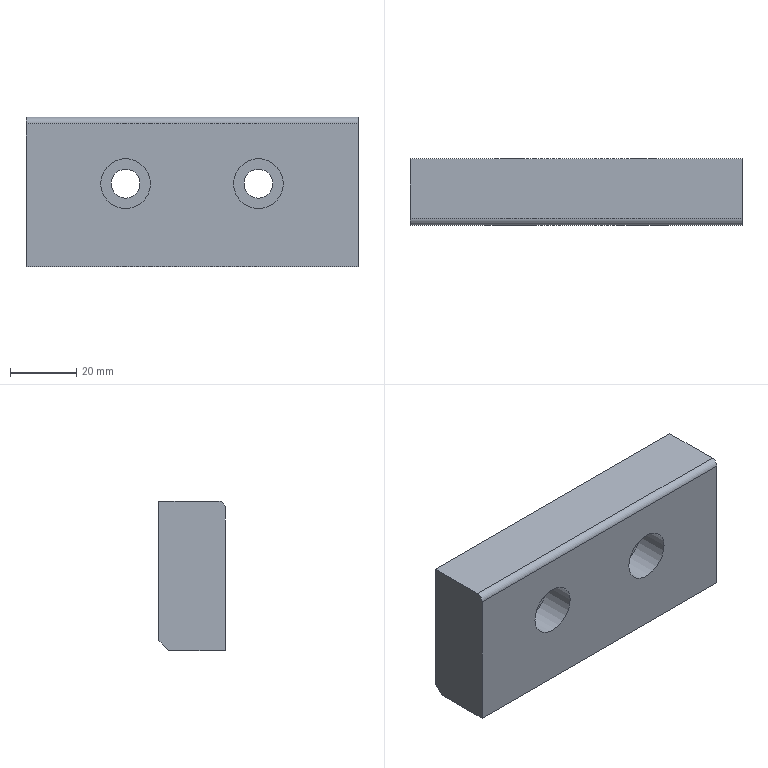Part | STEP file | 1_id1578_x_t | 1 solid | 14 faces | box 100 x 20 x 45 mm | volume 84741 mm3 | plane 9 | cylinder 5 | commonest cylinder face diameters 8.7 x2 15 x2 4 x1
STEP:
#1=CARTESIAN_POINT('',(0.,0.,0.));
#2=DIRECTION('',(0.,0.,1.));
#3=DIRECTION('',(1.,0.,0.));
#4=AXIS2_PLACEMENT_3D('',#1,#2,#3);
#5=CARTESIAN_POINT('',(797.926,444.972,-87.248));
#6=VERTEX_POINT('',#5);
#7=CARTESIAN_POINT('',(697.926,444.972,-87.248));
#8=VERTEX_POINT('',#7);
#9=CARTESIAN_POINT('',(797.926,444.972,-87.248));
#10=DIRECTION('',(-1.,0.,0.));
#11=VECTOR('',#10,1.);
#12=LINE('',#9,#11);
#13=CARTESIAN_POINT('',(707.926,444.972,-87.248));
#14=DIRECTION('',(0.,0.7071,-0.7071));
#15=DIRECTION('',(0.,-0.7071,-0.7071));
#16=AXIS2_PLACEMENT_3D('',#13,#14,#15);
#17=PLANE('',#16);
#18=CARTESIAN_POINT('',(0.,-90.));
#19=DIRECTION('',(0.,1.));
#20=VECTOR('',#19,1.);
#21=LINE('',#18,#20);
#22=(GEOMETRIC_REPRESENTATION_CONTEXT(2)PARAMETRIC_REPRESENTATION_CONTEXT()REPRESENTATION_CONTEXT('',''));
#23=DEFINITIONAL_REPRESENTATION('',(#21),#22);
#24=PCURVE('',#17,#23);
#25=CARTESIAN_POINT('',(707.926,444.972,-107.548));
#26=DIRECTION('',(0.,1.,0.));
#27=DIRECTION('',(1.,0.,0.));
#28=AXIS2_PLACEMENT_3D('',#25,#26,#27);
#29=PLANE('',#28);
#30=CARTESIAN_POINT('',(90.,-20.3));
#31=DIRECTION('',(-1.,0.));
#32=VECTOR('',#31,1.);
#33=LINE('',#30,#32);
#34=(GEOMETRIC_REPRESENTATION_CONTEXT(2)PARAMETRIC_REPRESENTATION_CONTEXT()REPRESENTATION_CONTEXT('',''));
#35=DEFINITIONAL_REPRESENTATION('',(#33),#34);
#36=PCURVE('',#29,#35);
#37=SURFACE_CURVE('',#12,(#24,#36),.PCURVE_S1.);
#38=EDGE_CURVE('',#6,#8,#37,.T.);
#39=ORIENTED_EDGE('',*,*,#38,.F.);
#40=CARTESIAN_POINT('',(797.926,441.972,-90.248));
#41=VERTEX_POINT('',#40);
#42=CARTESIAN_POINT('',(797.926,441.972,-90.248));
#43=DIRECTION('',(0.,0.7071,0.7071));
#44=VECTOR('',#43,1.);
#45=LINE('',#42,#44);
#46=CARTESIAN_POINT('',(4.243,-90.));
#47=DIRECTION('',(-1.,0.));
#48=VECTOR('',#47,1.);
#49=LINE('',#46,#48);
#50=(GEOMETRIC_REPRESENTATION_CONTEXT(2)PARAMETRIC_REPRESENTATION_CONTEXT()REPRESENTATION_CONTEXT('',''));
#51=DEFINITIONAL_REPRESENTATION('',(#49),#50);
#52=PCURVE('',#17,#51);
#53=CARTESIAN_POINT('',(797.926,544.972,-45.248));
#54=DIRECTION('',(-1.,0.,0.));
#55=DIRECTION('',(0.,0.,-1.));
#56=AXIS2_PLACEMENT_3D('',#53,#54,#55);
#57=PLANE('',#56);
#58=CARTESIAN_POINT('',(45.,103.));
#59=DIRECTION('',(-0.7071,-0.7071));
#60=VECTOR('',#59,1.);
#61=LINE('',#58,#60);
#62=(GEOMETRIC_REPRESENTATION_CONTEXT(2)PARAMETRIC_REPRESENTATION_CONTEXT()REPRESENTATION_CONTEXT('',''));
#63=DEFINITIONAL_REPRESENTATION('',(#61),#62);
#64=PCURVE('',#57,#63);
#65=SURFACE_CURVE('',#45,(#52,#64),.PCURVE_S1.);
#66=EDGE_CURVE('',#41,#6,#65,.T.);
#67=ORIENTED_EDGE('',*,*,#66,.F.);
#68=CARTESIAN_POINT('',(697.926,441.972,-90.248));
#69=VERTEX_POINT('',#68);
#70=CARTESIAN_POINT('',(697.926,441.972,-90.248));
#71=DIRECTION('',(1.,0.,0.));
#72=VECTOR('',#71,1.);
#73=LINE('',#70,#72);
#74=CARTESIAN_POINT('',(4.243,10.));
#75=DIRECTION('',(0.,-1.));
#76=VECTOR('',#75,1.);
#77=LINE('',#74,#76);
#78=(GEOMETRIC_REPRESENTATION_CONTEXT(2)PARAMETRIC_REPRESENTATION_CONTEXT()REPRESENTATION_CONTEXT('',''));
#79=DEFINITIONAL_REPRESENTATION('',(#77),#78);
#80=PCURVE('',#17,#79);
#81=CARTESIAN_POINT('',(787.926,424.972,-90.248));
#82=DIRECTION('',(0.,0.,1.));
#83=DIRECTION('',(-1.,0.,0.));
#84=AXIS2_PLACEMENT_3D('',#81,#82,#83);
#85=PLANE('',#84);
#86=CARTESIAN_POINT('',(90.,-17.));
#87=DIRECTION('',(-1.,0.));
#88=VECTOR('',#87,1.);
#89=LINE('',#86,#88);
#90=(GEOMETRIC_REPRESENTATION_CONTEXT(2)PARAMETRIC_REPRESENTATION_CONTEXT()REPRESENTATION_CONTEXT('',''));
#91=DEFINITIONAL_REPRESENTATION('',(#89),#90);
#92=PCURVE('',#85,#91);
#93=SURFACE_CURVE('',#73,(#80,#92),.PCURVE_S1.);
#94=EDGE_CURVE('',#69,#41,#93,.T.);
#95=ORIENTED_EDGE('',*,*,#94,.F.);
#96=CARTESIAN_POINT('',(697.926,444.972,-87.248));
#97=DIRECTION('',(0.,-0.7071,-0.7071));
#98=VECTOR('',#97,1.);
#99=LINE('',#96,#98);
#100=CARTESIAN_POINT('',(0.,10.));
#101=DIRECTION('',(1.,0.));
#102=VECTOR('',#101,1.);
#103=LINE('',#100,#102);
#104=(GEOMETRIC_REPRESENTATION_CONTEXT(2)PARAMETRIC_REPRESENTATION_CONTEXT()REPRESENTATION_CONTEXT('',''));
#105=DEFINITIONAL_REPRESENTATION('',(#103),#104);
#106=PCURVE('',#17,#105);
#107=CARTESIAN_POINT('',(697.926,444.972,-45.248));
#108=DIRECTION('',(1.,0.,0.));
#109=DIRECTION('',(0.,0.,-1.));
#110=AXIS2_PLACEMENT_3D('',#107,#108,#109);
#111=PLANE('',#110);
#112=CARTESIAN_POINT('',(42.,0.));
#113=DIRECTION('',(0.7071,-0.7071));
#114=VECTOR('',#113,1.);
#115=LINE('',#112,#114);
#116=(GEOMETRIC_REPRESENTATION_CONTEXT(2)PARAMETRIC_REPRESENTATION_CONTEXT()REPRESENTATION_CONTEXT('',''));
#117=DEFINITIONAL_REPRESENTATION('',(#115),#116);
#118=PCURVE('',#111,#117);
#119=SURFACE_CURVE('',#99,(#106,#118),.PCURVE_S1.);
#120=EDGE_CURVE('',#8,#69,#119,.T.);
#121=ORIENTED_EDGE('',*,*,#120,.F.);
#122=EDGE_LOOP('',(#39,#67,#95,#121));
#123=FACE_BOUND('',#122,.T.);
#124=ADVANCED_FACE('',(#123),#17,.T.);
#125=CARTESIAN_POINT('',(697.926,424.972,-47.248));
#126=VERTEX_POINT('',#125);
#127=CARTESIAN_POINT('',(697.926,424.972,-90.248));
#128=VERTEX_POINT('',#127);
#129=CARTESIAN_POINT('',(697.926,424.972,-47.248));
#130=DIRECTION('',(0.,0.,-1.));
#131=VECTOR('',#130,1.);
#132=LINE('',#129,#131);
#133=CARTESIAN_POINT('',(2.,-20.));
#134=DIRECTION('',(1.,0.));
#135=VECTOR('',#134,1.);
#136=LINE('',#133,#135);
#137=(GEOMETRIC_REPRESENTATION_CONTEXT(2)PARAMETRIC_REPRESENTATION_CONTEXT()REPRESENTATION_CONTEXT('',''));
#138=DEFINITIONAL_REPRESENTATION('',(#136),#137);
#139=PCURVE('',#111,#138);
#140=CARTESIAN_POINT('',(787.926,424.972,-107.548));
#141=DIRECTION('',(0.,-1.,0.));
#142=DIRECTION('',(-1.,0.,0.));
#143=AXIS2_PLACEMENT_3D('',#140,#141,#142);
#144=PLANE('',#143);
#145=CARTESIAN_POINT('',(90.,-60.3));
#146=DIRECTION('',(0.,1.));
#147=VECTOR('',#146,1.);
#148=LINE('',#145,#147);
#149=(GEOMETRIC_REPRESENTATION_CONTEXT(2)PARAMETRIC_REPRESENTATION_CONTEXT()REPRESENTATION_CONTEXT('',''));
#150=DEFINITIONAL_REPRESENTATION('',(#148),#149);
#151=PCURVE('',#144,#150);
#152=SURFACE_CURVE('',#132,(#139,#151),.PCURVE_S1.);
#153=EDGE_CURVE('',#126,#128,#152,.T.);
#154=ORIENTED_EDGE('',*,*,#153,.F.);
#155=CARTESIAN_POINT('',(697.926,426.972,-45.248));
#156=VERTEX_POINT('',#155);
#157=CARTESIAN_POINT('',(697.926,426.972,-47.248));
#158=DIRECTION('',(-1.,0.,0.));
#159=DIRECTION('',(0.,-1.,0.));
#160=AXIS2_PLACEMENT_3D('',#157,#158,#159);
#161=CIRCLE('',#160,2.);
#162=CARTESIAN_POINT('',(2.,-20.));
#163=CARTESIAN_POINT('',(-1.464,-20.));
#164=CARTESIAN_POINT('',(0.2679,-17.));
#165=CARTESIAN_POINT('',(2.,-14.));
#166=CARTESIAN_POINT('',(3.732,-17.));
#167=CARTESIAN_POINT('',(5.464,-20.));
#168=CARTESIAN_POINT('',(2.,-20.));
#169=(BOUNDED_CURVE()B_SPLINE_CURVE(2,(#162,#163,#164,#165,#166,#167,#168),.UNSPECIFIED.,.T.,.F.)B_SPLINE_CURVE_WITH_KNOTS((1,2,2,2,2,1),(-2.094,0.,2.094,4.189,6.283,8.378),.UNSPECIFIED.)CURVE()GEOMETRIC_REPRESENTATION_ITEM()RATIONAL_B_SPLINE_CURVE((1.,0.5,1.,0.5,1.,0.5,1.))REPRESENTATION_ITEM(''));
#170=(GEOMETRIC_REPRESENTATION_CONTEXT(2)PARAMETRIC_REPRESENTATION_CONTEXT()REPRESENTATION_CONTEXT('',''));
#171=DEFINITIONAL_REPRESENTATION('',(#169),#170);
#172=PCURVE('',#111,#171);
#173=CARTESIAN_POINT('',(787.926,426.972,-47.248));
#174=DIRECTION('',(1.,0.,0.));
#175=DIRECTION('',(0.,1.,0.));
#176=AXIS2_PLACEMENT_3D('',#173,#174,#175);
#177=CYLINDRICAL_SURFACE('',#176,2.);
#178=CARTESIAN_POINT('',(3.142,-90.));
#179=DIRECTION('',(-1.,0.));
#180=VECTOR('',#179,1.);
#181=LINE('',#178,#180);
#182=(GEOMETRIC_REPRESENTATION_CONTEXT(2)PARAMETRIC_REPRESENTATION_CONTEXT()REPRESENTATION_CONTEXT('',''));
#183=DEFINITIONAL_REPRESENTATION('',(#181),#182);
#184=PCURVE('',#177,#183);
#185=SURFACE_CURVE('',#161,(#172,#184),.PCURVE_S1.);
#186=EDGE_CURVE('',#126,#156,#185,.T.);
#187=ORIENTED_EDGE('',*,*,#186,.T.);
#188=CARTESIAN_POINT('',(697.926,444.972,-45.248));
#189=VERTEX_POINT('',#188);
#190=CARTESIAN_POINT('',(697.926,444.972,-45.248));
#191=DIRECTION('',(0.,-1.,0.));
#192=VECTOR('',#191,1.);
#193=LINE('',#190,#192);
#194=CARTESIAN_POINT('',(0.,0.));
#195=DIRECTION('',(0.,-1.));
#196=VECTOR('',#195,1.);
#197=LINE('',#194,#196);
#198=(GEOMETRIC_REPRESENTATION_CONTEXT(2)PARAMETRIC_REPRESENTATION_CONTEXT()REPRESENTATION_CONTEXT('',''));
#199=DEFINITIONAL_REPRESENTATION('',(#197),#198);
#200=PCURVE('',#111,#199);
#201=CARTESIAN_POINT('',(797.926,444.972,-45.248));
#202=DIRECTION('',(0.,0.,1.));
#203=DIRECTION('',(-1.,0.,0.));
#204=AXIS2_PLACEMENT_3D('',#201,#202,#203);
#205=PLANE('',#204);
#206=CARTESIAN_POINT('',(100.,0.));
#207=DIRECTION('',(0.,1.));
#208=VECTOR('',#207,1.);
#209=LINE('',#206,#208);
#210=(GEOMETRIC_REPRESENTATION_CONTEXT(2)PARAMETRIC_REPRESENTATION_CONTEXT()REPRESENTATION_CONTEXT('',''));
#211=DEFINITIONAL_REPRESENTATION('',(#209),#210);
#212=PCURVE('',#205,#211);
#213=SURFACE_CURVE('',#193,(#200,#212),.PCURVE_S1.);
#214=EDGE_CURVE('',#189,#156,#213,.T.);
#215=ORIENTED_EDGE('',*,*,#214,.F.);
#216=CARTESIAN_POINT('',(697.926,444.972,-45.248));
#217=DIRECTION('',(0.,0.,-1.));
#218=VECTOR('',#217,1.);
#219=LINE('',#216,#218);
#220=CARTESIAN_POINT('',(0.,0.));
#221=DIRECTION('',(1.,0.));
#222=VECTOR('',#221,1.);
#223=LINE('',#220,#222);
#224=(GEOMETRIC_REPRESENTATION_CONTEXT(2)PARAMETRIC_REPRESENTATION_CONTEXT()REPRESENTATION_CONTEXT('',''));
#225=DEFINITIONAL_REPRESENTATION('',(#223),#224);
#226=PCURVE('',#111,#225);
#227=CARTESIAN_POINT('',(-10.,-62.3));
#228=DIRECTION('',(0.,1.));
#229=VECTOR('',#228,1.);
#230=LINE('',#227,#229);
#231=(GEOMETRIC_REPRESENTATION_CONTEXT(2)PARAMETRIC_REPRESENTATION_CONTEXT()REPRESENTATION_CONTEXT('',''));
#232=DEFINITIONAL_REPRESENTATION('',(#230),#231);
#233=PCURVE('',#29,#232);
#234=SURFACE_CURVE('',#219,(#226,#233),.PCURVE_S1.);
#235=EDGE_CURVE('',#189,#8,#234,.T.);
#236=ORIENTED_EDGE('',*,*,#235,.T.);
#237=ORIENTED_EDGE('',*,*,#120,.T.);
#238=CARTESIAN_POINT('',(697.926,441.972,-90.248));
#239=DIRECTION('',(0.,-1.,0.));
#240=VECTOR('',#239,1.);
#241=LINE('',#238,#240);
#242=CARTESIAN_POINT('',(45.,-3.));
#243=DIRECTION('',(0.,-1.));
#244=VECTOR('',#243,1.);
#245=LINE('',#242,#244);
#246=(GEOMETRIC_REPRESENTATION_CONTEXT(2)PARAMETRIC_REPRESENTATION_CONTEXT()REPRESENTATION_CONTEXT('',''));
#247=DEFINITIONAL_REPRESENTATION('',(#245),#246);
#248=PCURVE('',#111,#247);
#249=CARTESIAN_POINT('',(90.,-17.));
#250=DIRECTION('',(0.,1.));
#251=VECTOR('',#250,1.);
#252=LINE('',#249,#251);
#253=(GEOMETRIC_REPRESENTATION_CONTEXT(2)PARAMETRIC_REPRESENTATION_CONTEXT()REPRESENTATION_CONTEXT('',''));
#254=DEFINITIONAL_REPRESENTATION('',(#252),#253);
#255=PCURVE('',#85,#254);
#256=SURFACE_CURVE('',#241,(#248,#255),.PCURVE_S1.);
#257=EDGE_CURVE('',#69,#128,#256,.T.);
#258=ORIENTED_EDGE('',*,*,#257,.T.);
#259=EDGE_LOOP('',(#154,#187,#215,#236,#237,#258));
#260=FACE_BOUND('',#259,.T.);
#261=ADVANCED_FACE('',(#260),#111,.F.);
#262=CARTESIAN_POINT('',(797.926,424.972,-90.248));
#263=VERTEX_POINT('',#262);
#264=CARTESIAN_POINT('',(697.926,424.972,-90.248));
#265=DIRECTION('',(1.,0.,0.));
#266=VECTOR('',#265,1.);
#267=LINE('',#264,#266);
#268=CARTESIAN_POINT('',(90.,0.));
#269=DIRECTION('',(-1.,0.));
#270=VECTOR('',#269,1.);
#271=LINE('',#268,#270);
#272=(GEOMETRIC_REPRESENTATION_CONTEXT(2)PARAMETRIC_REPRESENTATION_CONTEXT()REPRESENTATION_CONTEXT('',''));
#273=DEFINITIONAL_REPRESENTATION('',(#271),#272);
#274=PCURVE('',#85,#273);
#275=CARTESIAN_POINT('',(90.,-17.3));
#276=DIRECTION('',(-1.,0.));
#277=VECTOR('',#276,1.);
#278=LINE('',#275,#277);
#279=(GEOMETRIC_REPRESENTATION_CONTEXT(2)PARAMETRIC_REPRESENTATION_CONTEXT()REPRESENTATION_CONTEXT('',''));
#280=DEFINITIONAL_REPRESENTATION('',(#278),#279);
#281=PCURVE('',#144,#280);
#282=SURFACE_CURVE('',#267,(#274,#281),.PCURVE_S1.);
#283=EDGE_CURVE('',#128,#263,#282,.T.);
#284=ORIENTED_EDGE('',*,*,#283,.F.);
#285=ORIENTED_EDGE('',*,*,#257,.F.);
#286=ORIENTED_EDGE('',*,*,#94,.T.);
#287=CARTESIAN_POINT('',(797.926,424.972,-90.248));
#288=DIRECTION('',(0.,1.,0.));
#289=VECTOR('',#288,1.);
#290=LINE('',#287,#289);
#291=CARTESIAN_POINT('',(-10.,0.));
#292=DIRECTION('',(0.,-1.));
#293=VECTOR('',#292,1.);
#294=LINE('',#291,#293);
#295=(GEOMETRIC_REPRESENTATION_CONTEXT(2)PARAMETRIC_REPRESENTATION_CONTEXT()REPRESENTATION_CONTEXT('',''));
#296=DEFINITIONAL_REPRESENTATION('',(#294),#295);
#297=PCURVE('',#85,#296);
#298=CARTESIAN_POINT('',(45.,120.));
#299=DIRECTION('',(0.,-1.));
#300=VECTOR('',#299,1.);
#301=LINE('',#298,#300);
#302=(GEOMETRIC_REPRESENTATION_CONTEXT(2)PARAMETRIC_REPRESENTATION_CONTEXT()REPRESENTATION_CONTEXT('',''));
#303=DEFINITIONAL_REPRESENTATION('',(#301),#302);
#304=PCURVE('',#57,#303);
#305=SURFACE_CURVE('',#290,(#297,#304),.PCURVE_S1.);
#306=EDGE_CURVE('',#263,#41,#305,.T.);
#307=ORIENTED_EDGE('',*,*,#306,.F.);
#308=EDGE_LOOP('',(#284,#285,#286,#307));
#309=FACE_BOUND('',#308,.T.);
#310=ADVANCED_FACE('',(#309),#85,.F.);
#311=CARTESIAN_POINT('',(797.926,426.972,-45.248));
#312=VERTEX_POINT('',#311);
#313=CARTESIAN_POINT('',(797.926,444.972,-45.248));
#314=VERTEX_POINT('',#313);
#315=CARTESIAN_POINT('',(797.926,426.972,-45.248));
#316=DIRECTION('',(0.,1.,0.));
#317=VECTOR('',#316,1.);
#318=LINE('',#315,#317);
#319=CARTESIAN_POINT('',(0.,118.));
#320=DIRECTION('',(0.,-1.));
#321=VECTOR('',#320,1.);
#322=LINE('',#319,#321);
#323=(GEOMETRIC_REPRESENTATION_CONTEXT(2)PARAMETRIC_REPRESENTATION_CONTEXT()REPRESENTATION_CONTEXT('',''));
#324=DEFINITIONAL_REPRESENTATION('',(#322),#323);
#325=PCURVE('',#57,#324);
#326=CARTESIAN_POINT('',(0.,18.));
#327=DIRECTION('',(0.,-1.));
#328=VECTOR('',#327,1.);
#329=LINE('',#326,#328);
#330=(GEOMETRIC_REPRESENTATION_CONTEXT(2)PARAMETRIC_REPRESENTATION_CONTEXT()REPRESENTATION_CONTEXT('',''));
#331=DEFINITIONAL_REPRESENTATION('',(#329),#330);
#332=PCURVE('',#205,#331);
#333=SURFACE_CURVE('',#318,(#325,#332),.PCURVE_S1.);
#334=EDGE_CURVE('',#312,#314,#333,.T.);
#335=ORIENTED_EDGE('',*,*,#334,.F.);
#336=CARTESIAN_POINT('',(797.926,424.972,-47.248));
#337=VERTEX_POINT('',#336);
#338=CARTESIAN_POINT('',(797.926,426.972,-47.248));
#339=DIRECTION('',(1.,0.,0.));
#340=DIRECTION('',(0.,0.,1.));
#341=AXIS2_PLACEMENT_3D('',#338,#339,#340);
#342=CIRCLE('',#341,2.);
#343=CARTESIAN_POINT('',(0.,118.));
#344=CARTESIAN_POINT('',(0.,121.464));
#345=CARTESIAN_POINT('',(3.,119.732));
#346=CARTESIAN_POINT('',(6.,118.));
#347=CARTESIAN_POINT('',(3.,116.268));
#348=CARTESIAN_POINT('',(0.,114.536));
#349=CARTESIAN_POINT('',(0.,118.));
#350=(BOUNDED_CURVE()B_SPLINE_CURVE(2,(#343,#344,#345,#346,#347,#348,#349),.UNSPECIFIED.,.T.,.F.)B_SPLINE_CURVE_WITH_KNOTS((1,2,2,2,2,1),(-2.094,0.,2.094,4.189,6.283,8.378),.UNSPECIFIED.)CURVE()GEOMETRIC_REPRESENTATION_ITEM()RATIONAL_B_SPLINE_CURVE((1.,0.5,1.,0.5,1.,0.5,1.))REPRESENTATION_ITEM(''));
#351=(GEOMETRIC_REPRESENTATION_CONTEXT(2)PARAMETRIC_REPRESENTATION_CONTEXT()REPRESENTATION_CONTEXT('',''));
#352=DEFINITIONAL_REPRESENTATION('',(#350),#351);
#353=PCURVE('',#57,#352);
#354=CARTESIAN_POINT('',(1.571,10.));
#355=DIRECTION('',(1.,0.));
#356=VECTOR('',#355,1.);
#357=LINE('',#354,#356);
#358=(GEOMETRIC_REPRESENTATION_CONTEXT(2)PARAMETRIC_REPRESENTATION_CONTEXT()REPRESENTATION_CONTEXT('',''));
#359=DEFINITIONAL_REPRESENTATION('',(#357),#358);
#360=PCURVE('',#177,#359);
#361=SURFACE_CURVE('',#342,(#353,#360),.PCURVE_S1.);
#362=EDGE_CURVE('',#312,#337,#361,.T.);
#363=ORIENTED_EDGE('',*,*,#362,.T.);
#364=CARTESIAN_POINT('',(797.926,424.972,-47.248));
#365=DIRECTION('',(0.,0.,-1.));
#366=VECTOR('',#365,1.);
#367=LINE('',#364,#366);
#368=CARTESIAN_POINT('',(2.,120.));
#369=DIRECTION('',(1.,0.));
#370=VECTOR('',#369,1.);
#371=LINE('',#368,#370);
#372=(GEOMETRIC_REPRESENTATION_CONTEXT(2)PARAMETRIC_REPRESENTATION_CONTEXT()REPRESENTATION_CONTEXT('',''));
#373=DEFINITIONAL_REPRESENTATION('',(#371),#372);
#374=PCURVE('',#57,#373);
#375=CARTESIAN_POINT('',(-10.,-60.3));
#376=DIRECTION('',(0.,1.));
#377=VECTOR('',#376,1.);
#378=LINE('',#375,#377);
#379=(GEOMETRIC_REPRESENTATION_CONTEXT(2)PARAMETRIC_REPRESENTATION_CONTEXT()REPRESENTATION_CONTEXT('',''));
#380=DEFINITIONAL_REPRESENTATION('',(#378),#379);
#381=PCURVE('',#144,#380);
#382=SURFACE_CURVE('',#367,(#374,#381),.PCURVE_S1.);
#383=EDGE_CURVE('',#337,#263,#382,.T.);
#384=ORIENTED_EDGE('',*,*,#383,.T.);
#385=ORIENTED_EDGE('',*,*,#306,.T.);
#386=ORIENTED_EDGE('',*,*,#66,.T.);
#387=CARTESIAN_POINT('',(797.926,444.972,-45.248));
#388=DIRECTION('',(0.,0.,-1.));
#389=VECTOR('',#388,1.);
#390=LINE('',#387,#389);
#391=CARTESIAN_POINT('',(0.,100.));
#392=DIRECTION('',(1.,0.));
#393=VECTOR('',#392,1.);
#394=LINE('',#391,#393);
#395=(GEOMETRIC_REPRESENTATION_CONTEXT(2)PARAMETRIC_REPRESENTATION_CONTEXT()REPRESENTATION_CONTEXT('',''));
#396=DEFINITIONAL_REPRESENTATION('',(#394),#395);
#397=PCURVE('',#57,#396);
#398=CARTESIAN_POINT('',(90.,-62.3));
#399=DIRECTION('',(0.,1.));
#400=VECTOR('',#399,1.);
#401=LINE('',#398,#400);
#402=(GEOMETRIC_REPRESENTATION_CONTEXT(2)PARAMETRIC_REPRESENTATION_CONTEXT()REPRESENTATION_CONTEXT('',''));
#403=DEFINITIONAL_REPRESENTATION('',(#401),#402);
#404=PCURVE('',#29,#403);
#405=SURFACE_CURVE('',#390,(#397,#404),.PCURVE_S1.);
#406=EDGE_CURVE('',#314,#6,#405,.T.);
#407=ORIENTED_EDGE('',*,*,#406,.F.);
#408=EDGE_LOOP('',(#335,#363,#384,#385,#386,#407));
#409=FACE_BOUND('',#408,.T.);
#410=ADVANCED_FACE('',(#409),#57,.F.);
#411=CARTESIAN_POINT('',(797.926,444.972,-45.248));
#412=DIRECTION('',(-1.,0.,0.));
#413=VECTOR('',#412,1.);
#414=LINE('',#411,#413);
#415=CARTESIAN_POINT('',(90.,-62.3));
#416=DIRECTION('',(-1.,0.));
#417=VECTOR('',#416,1.);
#418=LINE('',#415,#417);
#419=(GEOMETRIC_REPRESENTATION_CONTEXT(2)PARAMETRIC_REPRESENTATION_CONTEXT()REPRESENTATION_CONTEXT('',''));
#420=DEFINITIONAL_REPRESENTATION('',(#418),#419);
#421=PCURVE('',#29,#420);
#422=CARTESIAN_POINT('',(0.,0.));
#423=DIRECTION('',(1.,0.));
#424=VECTOR('',#423,1.);
#425=LINE('',#422,#424);
#426=(GEOMETRIC_REPRESENTATION_CONTEXT(2)PARAMETRIC_REPRESENTATION_CONTEXT()REPRESENTATION_CONTEXT('',''));
#427=DEFINITIONAL_REPRESENTATION('',(#425),#426);
#428=PCURVE('',#205,#427);
#429=SURFACE_CURVE('',#414,(#421,#428),.PCURVE_S1.);
#430=EDGE_CURVE('',#314,#189,#429,.T.);
#431=ORIENTED_EDGE('',*,*,#430,.F.);
#432=ORIENTED_EDGE('',*,*,#406,.T.);
#433=ORIENTED_EDGE('',*,*,#38,.T.);
#434=ORIENTED_EDGE('',*,*,#235,.F.);
#435=EDGE_LOOP('',(#431,#432,#433,#434));
#436=FACE_BOUND('',#435,.T.);
#437=CARTESIAN_POINT('',(727.926,444.972,-60.898));
#438=VERTEX_POINT('',#437);
#439=CARTESIAN_POINT('',(727.926,444.972,-65.248));
#440=DIRECTION('',(0.,-1.,0.));
#441=DIRECTION('',(0.,0.,1.));
#442=AXIS2_PLACEMENT_3D('',#439,#440,#441);
#443=CIRCLE('',#442,4.35);
#444=CARTESIAN_POINT('',(20.,-46.65));
#445=CARTESIAN_POINT('',(12.466,-46.65));
#446=CARTESIAN_POINT('',(16.233,-40.125));
#447=CARTESIAN_POINT('',(20.,-33.6));
#448=CARTESIAN_POINT('',(23.767,-40.125));
#449=CARTESIAN_POINT('',(27.534,-46.65));
#450=CARTESIAN_POINT('',(20.,-46.65));
#451=(BOUNDED_CURVE()B_SPLINE_CURVE(2,(#444,#445,#446,#447,#448,#449,#450),.UNSPECIFIED.,.T.,.F.)B_SPLINE_CURVE_WITH_KNOTS((1,2,2,2,2,1),(-2.094,0.,2.094,4.189,6.283,8.378),.UNSPECIFIED.)CURVE()GEOMETRIC_REPRESENTATION_ITEM()RATIONAL_B_SPLINE_CURVE((1.,0.5,1.,0.5,1.,0.5,1.))REPRESENTATION_ITEM(''));
#452=(GEOMETRIC_REPRESENTATION_CONTEXT(2)PARAMETRIC_REPRESENTATION_CONTEXT()REPRESENTATION_CONTEXT('',''));
#453=DEFINITIONAL_REPRESENTATION('',(#451),#452);
#454=PCURVE('',#29,#453);
#455=CARTESIAN_POINT('',(727.926,445.172,-65.248));
#456=DIRECTION('',(0.,1.,0.));
#457=DIRECTION('',(-1.,0.,0.));
#458=AXIS2_PLACEMENT_3D('',#455,#456,#457);
#459=CYLINDRICAL_SURFACE('',#458,4.35);
#460=CARTESIAN_POINT('',(7.854,-0.2));
#461=DIRECTION('',(-1.,0.));
#462=VECTOR('',#461,1.);
#463=LINE('',#460,#462);
#464=(GEOMETRIC_REPRESENTATION_CONTEXT(2)PARAMETRIC_REPRESENTATION_CONTEXT()REPRESENTATION_CONTEXT('',''));
#465=DEFINITIONAL_REPRESENTATION('',(#463),#464);
#466=PCURVE('',#459,#465);
#467=SURFACE_CURVE('',#443,(#454,#466),.PCURVE_S1.);
#468=EDGE_CURVE('',#438,#438,#467,.T.);
#469=ORIENTED_EDGE('',*,*,#468,.T.);
#470=EDGE_LOOP('',(#469));
#471=FACE_BOUND('',#470,.T.);
#472=CARTESIAN_POINT('',(767.926,444.972,-60.898));
#473=VERTEX_POINT('',#472);
#474=CARTESIAN_POINT('',(767.926,444.972,-65.248));
#475=DIRECTION('',(0.,-1.,0.));
#476=DIRECTION('',(0.,0.,1.));
#477=AXIS2_PLACEMENT_3D('',#474,#475,#476);
#478=CIRCLE('',#477,4.35);
#479=CARTESIAN_POINT('',(60.,-46.65));
#480=CARTESIAN_POINT('',(52.466,-46.65));
#481=CARTESIAN_POINT('',(56.233,-40.125));
#482=CARTESIAN_POINT('',(60.,-33.6));
#483=CARTESIAN_POINT('',(63.767,-40.125));
#484=CARTESIAN_POINT('',(67.534,-46.65));
#485=CARTESIAN_POINT('',(60.,-46.65));
#486=(BOUNDED_CURVE()B_SPLINE_CURVE(2,(#479,#480,#481,#482,#483,#484,#485),.UNSPECIFIED.,.T.,.F.)B_SPLINE_CURVE_WITH_KNOTS((1,2,2,2,2,1),(-2.094,0.,2.094,4.189,6.283,8.378),.UNSPECIFIED.)CURVE()GEOMETRIC_REPRESENTATION_ITEM()RATIONAL_B_SPLINE_CURVE((1.,0.5,1.,0.5,1.,0.5,1.))REPRESENTATION_ITEM(''));
#487=(GEOMETRIC_REPRESENTATION_CONTEXT(2)PARAMETRIC_REPRESENTATION_CONTEXT()REPRESENTATION_CONTEXT('',''));
#488=DEFINITIONAL_REPRESENTATION('',(#486),#487);
#489=PCURVE('',#29,#488);
#490=CARTESIAN_POINT('',(767.926,445.172,-65.248));
#491=DIRECTION('',(0.,1.,0.));
#492=DIRECTION('',(-1.,0.,0.));
#493=AXIS2_PLACEMENT_3D('',#490,#491,#492);
#494=CYLINDRICAL_SURFACE('',#493,4.35);
#495=CARTESIAN_POINT('',(7.854,-0.2));
#496=DIRECTION('',(-1.,0.));
#497=VECTOR('',#496,1.);
#498=LINE('',#495,#497);
#499=(GEOMETRIC_REPRESENTATION_CONTEXT(2)PARAMETRIC_REPRESENTATION_CONTEXT()REPRESENTATION_CONTEXT('',''));
#500=DEFINITIONAL_REPRESENTATION('',(#498),#499);
#501=PCURVE('',#494,#500);
#502=SURFACE_CURVE('',#478,(#489,#501),.PCURVE_S1.);
#503=EDGE_CURVE('',#473,#473,#502,.T.);
#504=ORIENTED_EDGE('',*,*,#503,.T.);
#505=EDGE_LOOP('',(#504));
#506=FACE_BOUND('',#505,.T.);
#507=ADVANCED_FACE('',(#436,#471,#506),#29,.T.);
#508=ORIENTED_EDGE('',*,*,#430,.T.);
#509=ORIENTED_EDGE('',*,*,#214,.T.);
#510=CARTESIAN_POINT('',(797.926,426.972,-45.248));
#511=DIRECTION('',(-1.,0.,0.));
#512=VECTOR('',#511,1.);
#513=LINE('',#510,#512);
#514=CARTESIAN_POINT('',(0.,18.));
#515=DIRECTION('',(1.,0.));
#516=VECTOR('',#515,1.);
#517=LINE('',#514,#516);
#518=(GEOMETRIC_REPRESENTATION_CONTEXT(2)PARAMETRIC_REPRESENTATION_CONTEXT()REPRESENTATION_CONTEXT('',''));
#519=DEFINITIONAL_REPRESENTATION('',(#517),#518);
#520=PCURVE('',#205,#519);
#521=CARTESIAN_POINT('',(1.571,10.));
#522=DIRECTION('',(0.,-1.));
#523=VECTOR('',#522,1.);
#524=LINE('',#521,#523);
#525=(GEOMETRIC_REPRESENTATION_CONTEXT(2)PARAMETRIC_REPRESENTATION_CONTEXT()REPRESENTATION_CONTEXT('',''));
#526=DEFINITIONAL_REPRESENTATION('',(#524),#525);
#527=PCURVE('',#177,#526);
#528=SURFACE_CURVE('',#513,(#520,#527),.PCURVE_S1.);
#529=EDGE_CURVE('',#312,#156,#528,.T.);
#530=ORIENTED_EDGE('',*,*,#529,.F.);
#531=ORIENTED_EDGE('',*,*,#334,.T.);
#532=EDGE_LOOP('',(#508,#509,#530,#531));
#533=FACE_BOUND('',#532,.T.);
#534=ADVANCED_FACE('',(#533),#205,.T.);
#535=ORIENTED_EDGE('',*,*,#529,.T.);
#536=ORIENTED_EDGE('',*,*,#186,.F.);
#537=CARTESIAN_POINT('',(697.926,424.972,-47.248));
#538=DIRECTION('',(1.,0.,0.));
#539=VECTOR('',#538,1.);
#540=LINE('',#537,#539);
#541=CARTESIAN_POINT('',(3.142,-90.));
#542=DIRECTION('',(0.,1.));
#543=VECTOR('',#542,1.);
#544=LINE('',#541,#543);
#545=(GEOMETRIC_REPRESENTATION_CONTEXT(2)PARAMETRIC_REPRESENTATION_CONTEXT()REPRESENTATION_CONTEXT('',''));
#546=DEFINITIONAL_REPRESENTATION('',(#544),#545);
#547=PCURVE('',#177,#546);
#548=CARTESIAN_POINT('',(90.,-60.3));
#549=DIRECTION('',(-1.,0.));
#550=VECTOR('',#549,1.);
#551=LINE('',#548,#550);
#552=(GEOMETRIC_REPRESENTATION_CONTEXT(2)PARAMETRIC_REPRESENTATION_CONTEXT()REPRESENTATION_CONTEXT('',''));
#553=DEFINITIONAL_REPRESENTATION('',(#551),#552);
#554=PCURVE('',#144,#553);
#555=SURFACE_CURVE('',#540,(#547,#554),.PCURVE_S1.);
#556=EDGE_CURVE('',#126,#337,#555,.T.);
#557=ORIENTED_EDGE('',*,*,#556,.T.);
#558=ORIENTED_EDGE('',*,*,#362,.F.);
#559=EDGE_LOOP('',(#535,#536,#557,#558));
#560=FACE_BOUND('',#559,.T.);
#561=ADVANCED_FACE('',(#560),#177,.T.);
#562=ORIENTED_EDGE('',*,*,#283,.T.);
#563=ORIENTED_EDGE('',*,*,#383,.F.);
#564=ORIENTED_EDGE('',*,*,#556,.F.);
#565=ORIENTED_EDGE('',*,*,#153,.T.);
#566=EDGE_LOOP('',(#562,#563,#564,#565));
#567=FACE_BOUND('',#566,.T.);
#568=CARTESIAN_POINT('',(775.426,424.972,-65.248));
#569=VERTEX_POINT('',#568);
#570=CARTESIAN_POINT('',(760.426,424.972,-65.248));
#571=VERTEX_POINT('',#570);
#572=CARTESIAN_POINT('',(767.926,424.972,-65.248));
#573=DIRECTION('',(0.,1.,0.));
#574=DIRECTION('',(1.,0.,0.));
#575=AXIS2_PLACEMENT_3D('',#572,#573,#574);
#576=CIRCLE('',#575,7.5);
#577=CARTESIAN_POINT('',(12.5,-42.3));
#578=CARTESIAN_POINT('',(12.5,-29.31));
#579=CARTESIAN_POINT('',(23.75,-35.805));
#580=CARTESIAN_POINT('',(35.,-42.3));
#581=CARTESIAN_POINT('',(23.75,-48.795));
#582=CARTESIAN_POINT('',(12.5,-55.29));
#583=CARTESIAN_POINT('',(12.5,-42.3));
#584=(BOUNDED_CURVE()B_SPLINE_CURVE(2,(#577,#578,#579,#580,#581,#582,#583),.UNSPECIFIED.,.T.,.F.)B_SPLINE_CURVE_WITH_KNOTS((1,2,2,2,2,1),(-2.094,0.,2.094,4.189,6.283,8.378),.UNSPECIFIED.)CURVE()GEOMETRIC_REPRESENTATION_ITEM()RATIONAL_B_SPLINE_CURVE((1.,0.5,1.,0.5,1.,0.5,1.))REPRESENTATION_ITEM(''));
#585=(GEOMETRIC_REPRESENTATION_CONTEXT(2)PARAMETRIC_REPRESENTATION_CONTEXT()REPRESENTATION_CONTEXT('',''));
#586=DEFINITIONAL_REPRESENTATION('',(#584),#585);
#587=PCURVE('',#144,#586);
#588=CARTESIAN_POINT('',(767.926,434.972,-65.248));
#589=DIRECTION('',(0.,1.,0.));
#590=DIRECTION('',(-1.,0.,0.));
#591=AXIS2_PLACEMENT_3D('',#588,#589,#590);
#592=CYLINDRICAL_SURFACE('',#591,7.5);
#593=CARTESIAN_POINT('',(3.142,-10.));
#594=DIRECTION('',(1.,0.));
#595=VECTOR('',#594,1.);
#596=LINE('',#593,#595);
#597=(GEOMETRIC_REPRESENTATION_CONTEXT(2)PARAMETRIC_REPRESENTATION_CONTEXT()REPRESENTATION_CONTEXT('',''));
#598=DEFINITIONAL_REPRESENTATION('',(#596),#597);
#599=PCURVE('',#592,#598);
#600=SURFACE_CURVE('',#576,(#587,#599),.PCURVE_S1.);
#601=EDGE_CURVE('',#569,#571,#600,.T.);
#602=ORIENTED_EDGE('',*,*,#601,.T.);
#603=CARTESIAN_POINT('',(767.926,424.972,-65.248));
#604=DIRECTION('',(0.,1.,0.));
#605=DIRECTION('',(1.,0.,0.));
#606=AXIS2_PLACEMENT_3D('',#603,#604,#605);
#607=CIRCLE('',#606,7.5);
#608=CARTESIAN_POINT('',(12.5,-42.3));
#609=CARTESIAN_POINT('',(12.5,-29.31));
#610=CARTESIAN_POINT('',(23.75,-35.805));
#611=CARTESIAN_POINT('',(35.,-42.3));
#612=CARTESIAN_POINT('',(23.75,-48.795));
#613=CARTESIAN_POINT('',(12.5,-55.29));
#614=CARTESIAN_POINT('',(12.5,-42.3));
#615=(BOUNDED_CURVE()B_SPLINE_CURVE(2,(#608,#609,#610,#611,#612,#613,#614),.UNSPECIFIED.,.T.,.F.)B_SPLINE_CURVE_WITH_KNOTS((1,2,2,2,2,1),(-2.094,0.,2.094,4.189,6.283,8.378),.UNSPECIFIED.)CURVE()GEOMETRIC_REPRESENTATION_ITEM()RATIONAL_B_SPLINE_CURVE((1.,0.5,1.,0.5,1.,0.5,1.))REPRESENTATION_ITEM(''));
#616=(GEOMETRIC_REPRESENTATION_CONTEXT(2)PARAMETRIC_REPRESENTATION_CONTEXT()REPRESENTATION_CONTEXT('',''));
#617=DEFINITIONAL_REPRESENTATION('',(#615),#616);
#618=PCURVE('',#144,#617);
#619=CARTESIAN_POINT('',(-3.142,-10.));
#620=DIRECTION('',(1.,0.));
#621=VECTOR('',#620,1.);
#622=LINE('',#619,#621);
#623=(GEOMETRIC_REPRESENTATION_CONTEXT(2)PARAMETRIC_REPRESENTATION_CONTEXT()REPRESENTATION_CONTEXT('',''));
#624=DEFINITIONAL_REPRESENTATION('',(#622),#623);
#625=PCURVE('',#592,#624);
#626=SURFACE_CURVE('',#607,(#618,#625),.PCURVE_S1.);
#627=EDGE_CURVE('',#571,#569,#626,.T.);
#628=ORIENTED_EDGE('',*,*,#627,.T.);
#629=EDGE_LOOP('',(#602,#628));
#630=FACE_BOUND('',#629,.T.);
#631=CARTESIAN_POINT('',(735.426,424.972,-65.248));
#632=VERTEX_POINT('',#631);
#633=CARTESIAN_POINT('',(720.426,424.972,-65.248));
#634=VERTEX_POINT('',#633);
#635=CARTESIAN_POINT('',(727.926,424.972,-65.248));
#636=DIRECTION('',(0.,1.,0.));
#637=DIRECTION('',(1.,0.,0.));
#638=AXIS2_PLACEMENT_3D('',#635,#636,#637);
#639=CIRCLE('',#638,7.5);
#640=CARTESIAN_POINT('',(52.5,-42.3));
#641=CARTESIAN_POINT('',(52.5,-29.31));
#642=CARTESIAN_POINT('',(63.75,-35.805));
#643=CARTESIAN_POINT('',(75.,-42.3));
#644=CARTESIAN_POINT('',(63.75,-48.795));
#645=CARTESIAN_POINT('',(52.5,-55.29));
#646=CARTESIAN_POINT('',(52.5,-42.3));
#647=(BOUNDED_CURVE()B_SPLINE_CURVE(2,(#640,#641,#642,#643,#644,#645,#646),.UNSPECIFIED.,.T.,.F.)B_SPLINE_CURVE_WITH_KNOTS((1,2,2,2,2,1),(-2.094,0.,2.094,4.189,6.283,8.378),.UNSPECIFIED.)CURVE()GEOMETRIC_REPRESENTATION_ITEM()RATIONAL_B_SPLINE_CURVE((1.,0.5,1.,0.5,1.,0.5,1.))REPRESENTATION_ITEM(''));
#648=(GEOMETRIC_REPRESENTATION_CONTEXT(2)PARAMETRIC_REPRESENTATION_CONTEXT()REPRESENTATION_CONTEXT('',''));
#649=DEFINITIONAL_REPRESENTATION('',(#647),#648);
#650=PCURVE('',#144,#649);
#651=CARTESIAN_POINT('',(727.926,434.972,-65.248));
#652=DIRECTION('',(0.,1.,0.));
#653=DIRECTION('',(-1.,0.,0.));
#654=AXIS2_PLACEMENT_3D('',#651,#652,#653);
#655=CYLINDRICAL_SURFACE('',#654,7.5);
#656=CARTESIAN_POINT('',(3.142,-10.));
#657=DIRECTION('',(1.,0.));
#658=VECTOR('',#657,1.);
#659=LINE('',#656,#658);
#660=(GEOMETRIC_REPRESENTATION_CONTEXT(2)PARAMETRIC_REPRESENTATION_CONTEXT()REPRESENTATION_CONTEXT('',''));
#661=DEFINITIONAL_REPRESENTATION('',(#659),#660);
#662=PCURVE('',#655,#661);
#663=SURFACE_CURVE('',#639,(#650,#662),.PCURVE_S1.);
#664=EDGE_CURVE('',#632,#634,#663,.T.);
#665=ORIENTED_EDGE('',*,*,#664,.T.);
#666=CARTESIAN_POINT('',(727.926,424.972,-65.248));
#667=DIRECTION('',(0.,1.,0.));
#668=DIRECTION('',(1.,0.,0.));
#669=AXIS2_PLACEMENT_3D('',#666,#667,#668);
#670=CIRCLE('',#669,7.5);
#671=CARTESIAN_POINT('',(52.5,-42.3));
#672=CARTESIAN_POINT('',(52.5,-29.31));
#673=CARTESIAN_POINT('',(63.75,-35.805));
#674=CARTESIAN_POINT('',(75.,-42.3));
#675=CARTESIAN_POINT('',(63.75,-48.795));
#676=CARTESIAN_POINT('',(52.5,-55.29));
#677=CARTESIAN_POINT('',(52.5,-42.3));
#678=(BOUNDED_CURVE()B_SPLINE_CURVE(2,(#671,#672,#673,#674,#675,#676,#677),.UNSPECIFIED.,.T.,.F.)B_SPLINE_CURVE_WITH_KNOTS((1,2,2,2,2,1),(-2.094,0.,2.094,4.189,6.283,8.378),.UNSPECIFIED.)CURVE()GEOMETRIC_REPRESENTATION_ITEM()RATIONAL_B_SPLINE_CURVE((1.,0.5,1.,0.5,1.,0.5,1.))REPRESENTATION_ITEM(''));
#679=(GEOMETRIC_REPRESENTATION_CONTEXT(2)PARAMETRIC_REPRESENTATION_CONTEXT()REPRESENTATION_CONTEXT('',''));
#680=DEFINITIONAL_REPRESENTATION('',(#678),#679);
#681=PCURVE('',#144,#680);
#682=CARTESIAN_POINT('',(-3.142,-10.));
#683=DIRECTION('',(1.,0.));
#684=VECTOR('',#683,1.);
#685=LINE('',#682,#684);
#686=(GEOMETRIC_REPRESENTATION_CONTEXT(2)PARAMETRIC_REPRESENTATION_CONTEXT()REPRESENTATION_CONTEXT('',''));
#687=DEFINITIONAL_REPRESENTATION('',(#685),#686);
#688=PCURVE('',#655,#687);
#689=SURFACE_CURVE('',#670,(#681,#688),.PCURVE_S1.);
#690=EDGE_CURVE('',#634,#632,#689,.T.);
#691=ORIENTED_EDGE('',*,*,#690,.T.);
#692=EDGE_LOOP('',(#665,#691));
#693=FACE_BOUND('',#692,.T.);
#694=ADVANCED_FACE('',(#567,#630,#693),#144,.T.);
#695=CARTESIAN_POINT('',(760.426,434.972,-65.248));
#696=VERTEX_POINT('',#695);
#697=CARTESIAN_POINT('',(767.926,434.972,-65.248));
#698=DIRECTION('',(0.,-1.,0.));
#699=DIRECTION('',(-1.,0.,0.));
#700=AXIS2_PLACEMENT_3D('',#697,#698,#699);
#701=CIRCLE('',#700,7.5);
#702=CARTESIAN_POINT('',(6.283,0.));
#703=DIRECTION('',(-1.,0.));
#704=VECTOR('',#703,1.);
#705=LINE('',#702,#704);
#706=(GEOMETRIC_REPRESENTATION_CONTEXT(2)PARAMETRIC_REPRESENTATION_CONTEXT()REPRESENTATION_CONTEXT('',''));
#707=DEFINITIONAL_REPRESENTATION('',(#705),#706);
#708=PCURVE('',#592,#707);
#709=CARTESIAN_POINT('',(767.926,434.972,-65.248));
#710=DIRECTION('',(0.,1.,0.));
#711=DIRECTION('',(1.,0.,0.));
#712=AXIS2_PLACEMENT_3D('',#709,#710,#711);
#713=PLANE('',#712);
#714=CARTESIAN_POINT('',(-7.5,0.));
#715=CARTESIAN_POINT('',(-7.5,12.99));
#716=CARTESIAN_POINT('',(3.75,6.495));
#717=CARTESIAN_POINT('',(15.,0.));
#718=CARTESIAN_POINT('',(3.75,-6.495));
#719=CARTESIAN_POINT('',(-7.5,-12.99));
#720=CARTESIAN_POINT('',(-7.5,0.));
#721=(BOUNDED_CURVE()B_SPLINE_CURVE(2,(#714,#715,#716,#717,#718,#719,#720),.UNSPECIFIED.,.T.,.F.)B_SPLINE_CURVE_WITH_KNOTS((1,2,2,2,2,1),(-2.094,0.,2.094,4.189,6.283,8.378),.UNSPECIFIED.)CURVE()GEOMETRIC_REPRESENTATION_ITEM()RATIONAL_B_SPLINE_CURVE((1.,0.5,1.,0.5,1.,0.5,1.))REPRESENTATION_ITEM(''));
#722=(GEOMETRIC_REPRESENTATION_CONTEXT(2)PARAMETRIC_REPRESENTATION_CONTEXT()REPRESENTATION_CONTEXT('',''));
#723=DEFINITIONAL_REPRESENTATION('',(#721),#722);
#724=PCURVE('',#713,#723);
#725=SURFACE_CURVE('',#701,(#708,#724),.PCURVE_S1.);
#726=EDGE_CURVE('',#696,#696,#725,.T.);
#727=ORIENTED_EDGE('',*,*,#726,.T.);
#728=CARTESIAN_POINT('',(760.426,424.972,-65.248));
#729=CARTESIAN_POINT('',(760.426,434.972,-65.248));
#730=B_SPLINE_CURVE_WITH_KNOTS('',1,(#728,#729),.UNSPECIFIED.,.F.,.F.,(2,2),(-10.,0.),.PIECEWISE_BEZIER_KNOTS.);
#731=CARTESIAN_POINT('',(0.,0.));
#732=DIRECTION('',(0.,1.));
#733=VECTOR('',#732,1.);
#734=LINE('',#731,#733);
#735=(GEOMETRIC_REPRESENTATION_CONTEXT(2)PARAMETRIC_REPRESENTATION_CONTEXT()REPRESENTATION_CONTEXT('',''));
#736=DEFINITIONAL_REPRESENTATION('',(#734),#735);
#737=PCURVE('',#592,#736);
#738=CARTESIAN_POINT('',(6.283,0.));
#739=DIRECTION('',(0.,1.));
#740=VECTOR('',#739,1.);
#741=LINE('',#738,#740);
#742=(GEOMETRIC_REPRESENTATION_CONTEXT(2)PARAMETRIC_REPRESENTATION_CONTEXT()REPRESENTATION_CONTEXT('',''));
#743=DEFINITIONAL_REPRESENTATION('',(#741),#742);
#744=PCURVE('',#592,#743);
#745=SEAM_CURVE('',#730,(#737,#744),.PCURVE_S1.);
#746=EDGE_CURVE('',#571,#696,#745,.T.);
#747=ORIENTED_EDGE('',*,*,#746,.F.);
#748=ORIENTED_EDGE('',*,*,#627,.T.);
#749=ORIENTED_EDGE('',*,*,#601,.T.);
#750=ORIENTED_EDGE('',*,*,#746,.T.);
#751=EDGE_LOOP('',(#727,#747,#748,#749,#750));
#752=FACE_BOUND('',#751,.F.);
#753=ADVANCED_FACE('',(#752),#592,.F.);
#754=ORIENTED_EDGE('',*,*,#726,.T.);
#755=EDGE_LOOP('',(#754));
#756=FACE_BOUND('',#755,.T.);
#757=CARTESIAN_POINT('',(767.926,434.972,-60.898));
#758=VERTEX_POINT('',#757);
#759=CARTESIAN_POINT('',(767.926,434.972,-65.248));
#760=DIRECTION('',(0.,1.,0.));
#761=DIRECTION('',(0.,0.,1.));
#762=AXIS2_PLACEMENT_3D('',#759,#760,#761);
#763=CIRCLE('',#762,4.35);
#764=CARTESIAN_POINT('',(0.,0.));
#765=DIRECTION('',(0.,-1.));
#766=AXIS2_PLACEMENT_2D('',#764,#765);
#767=CIRCLE('',#766,4.35);
#768=(GEOMETRIC_REPRESENTATION_CONTEXT(2)PARAMETRIC_REPRESENTATION_CONTEXT()REPRESENTATION_CONTEXT('',''));
#769=DEFINITIONAL_REPRESENTATION('',(#767),#768);
#770=PCURVE('',#713,#769);
#771=CARTESIAN_POINT('',(1.571,-10.2));
#772=DIRECTION('',(1.,0.));
#773=VECTOR('',#772,1.);
#774=LINE('',#771,#773);
#775=(GEOMETRIC_REPRESENTATION_CONTEXT(2)PARAMETRIC_REPRESENTATION_CONTEXT()REPRESENTATION_CONTEXT('',''));
#776=DEFINITIONAL_REPRESENTATION('',(#774),#775);
#777=PCURVE('',#494,#776);
#778=SURFACE_CURVE('',#763,(#770,#777),.PCURVE_S1.);
#779=EDGE_CURVE('',#758,#758,#778,.T.);
#780=ORIENTED_EDGE('',*,*,#779,.T.);
#781=EDGE_LOOP('',(#780));
#782=FACE_BOUND('',#781,.T.);
#783=ADVANCED_FACE('',(#756,#782),#713,.F.);
#784=ORIENTED_EDGE('',*,*,#503,.T.);
#785=CARTESIAN_POINT('',(767.926,434.972,-60.898));
#786=CARTESIAN_POINT('',(767.926,444.972,-60.898));
#787=B_SPLINE_CURVE_WITH_KNOTS('',1,(#785,#786),.UNSPECIFIED.,.F.,.F.,(2,2),(-10.2,-0.2),.PIECEWISE_BEZIER_KNOTS.);
#788=CARTESIAN_POINT('',(1.571,0.));
#789=DIRECTION('',(0.,1.));
#790=VECTOR('',#789,1.);
#791=LINE('',#788,#790);
#792=(GEOMETRIC_REPRESENTATION_CONTEXT(2)PARAMETRIC_REPRESENTATION_CONTEXT()REPRESENTATION_CONTEXT('',''));
#793=DEFINITIONAL_REPRESENTATION('',(#791),#792);
#794=PCURVE('',#494,#793);
#795=CARTESIAN_POINT('',(7.854,0.));
#796=DIRECTION('',(0.,1.));
#797=VECTOR('',#796,1.);
#798=LINE('',#795,#797);
#799=(GEOMETRIC_REPRESENTATION_CONTEXT(2)PARAMETRIC_REPRESENTATION_CONTEXT()REPRESENTATION_CONTEXT('',''));
#800=DEFINITIONAL_REPRESENTATION('',(#798),#799);
#801=PCURVE('',#494,#800);
#802=SEAM_CURVE('',#787,(#794,#801),.PCURVE_S1.);
#803=EDGE_CURVE('',#758,#473,#802,.T.);
#804=ORIENTED_EDGE('',*,*,#803,.F.);
#805=ORIENTED_EDGE('',*,*,#779,.T.);
#806=ORIENTED_EDGE('',*,*,#803,.T.);
#807=EDGE_LOOP('',(#784,#804,#805,#806));
#808=FACE_BOUND('',#807,.F.);
#809=ADVANCED_FACE('',(#808),#494,.F.);
#810=CARTESIAN_POINT('',(720.426,434.972,-65.248));
#811=VERTEX_POINT('',#810);
#812=CARTESIAN_POINT('',(727.926,434.972,-65.248));
#813=DIRECTION('',(0.,-1.,0.));
#814=DIRECTION('',(-1.,0.,0.));
#815=AXIS2_PLACEMENT_3D('',#812,#813,#814);
#816=CIRCLE('',#815,7.5);
#817=CARTESIAN_POINT('',(6.283,0.));
#818=DIRECTION('',(-1.,0.));
#819=VECTOR('',#818,1.);
#820=LINE('',#817,#819);
#821=(GEOMETRIC_REPRESENTATION_CONTEXT(2)PARAMETRIC_REPRESENTATION_CONTEXT()REPRESENTATION_CONTEXT('',''));
#822=DEFINITIONAL_REPRESENTATION('',(#820),#821);
#823=PCURVE('',#655,#822);
#824=CARTESIAN_POINT('',(727.926,434.972,-65.248));
#825=DIRECTION('',(0.,1.,0.));
#826=DIRECTION('',(1.,0.,0.));
#827=AXIS2_PLACEMENT_3D('',#824,#825,#826);
#828=PLANE('',#827);
#829=CARTESIAN_POINT('',(-7.5,0.));
#830=CARTESIAN_POINT('',(-7.5,12.99));
#831=CARTESIAN_POINT('',(3.75,6.495));
#832=CARTESIAN_POINT('',(15.,0.));
#833=CARTESIAN_POINT('',(3.75,-6.495));
#834=CARTESIAN_POINT('',(-7.5,-12.99));
#835=CARTESIAN_POINT('',(-7.5,0.));
#836=(BOUNDED_CURVE()B_SPLINE_CURVE(2,(#829,#830,#831,#832,#833,#834,#835),.UNSPECIFIED.,.T.,.F.)B_SPLINE_CURVE_WITH_KNOTS((1,2,2,2,2,1),(-2.094,0.,2.094,4.189,6.283,8.378),.UNSPECIFIED.)CURVE()GEOMETRIC_REPRESENTATION_ITEM()RATIONAL_B_SPLINE_CURVE((1.,0.5,1.,0.5,1.,0.5,1.))REPRESENTATION_ITEM(''));
#837=(GEOMETRIC_REPRESENTATION_CONTEXT(2)PARAMETRIC_REPRESENTATION_CONTEXT()REPRESENTATION_CONTEXT('',''));
#838=DEFINITIONAL_REPRESENTATION('',(#836),#837);
#839=PCURVE('',#828,#838);
#840=SURFACE_CURVE('',#816,(#823,#839),.PCURVE_S1.);
#841=EDGE_CURVE('',#811,#811,#840,.T.);
#842=ORIENTED_EDGE('',*,*,#841,.T.);
#843=CARTESIAN_POINT('',(720.426,424.972,-65.248));
#844=CARTESIAN_POINT('',(720.426,434.972,-65.248));
#845=B_SPLINE_CURVE_WITH_KNOTS('',1,(#843,#844),.UNSPECIFIED.,.F.,.F.,(2,2),(-10.,0.),.PIECEWISE_BEZIER_KNOTS.);
#846=CARTESIAN_POINT('',(0.,0.));
#847=DIRECTION('',(0.,1.));
#848=VECTOR('',#847,1.);
#849=LINE('',#846,#848);
#850=(GEOMETRIC_REPRESENTATION_CONTEXT(2)PARAMETRIC_REPRESENTATION_CONTEXT()REPRESENTATION_CONTEXT('',''));
#851=DEFINITIONAL_REPRESENTATION('',(#849),#850);
#852=PCURVE('',#655,#851);
#853=CARTESIAN_POINT('',(6.283,0.));
#854=DIRECTION('',(0.,1.));
#855=VECTOR('',#854,1.);
#856=LINE('',#853,#855);
#857=(GEOMETRIC_REPRESENTATION_CONTEXT(2)PARAMETRIC_REPRESENTATION_CONTEXT()REPRESENTATION_CONTEXT('',''));
#858=DEFINITIONAL_REPRESENTATION('',(#856),#857);
#859=PCURVE('',#655,#858);
#860=SEAM_CURVE('',#845,(#852,#859),.PCURVE_S1.);
#861=EDGE_CURVE('',#634,#811,#860,.T.);
#862=ORIENTED_EDGE('',*,*,#861,.F.);
#863=ORIENTED_EDGE('',*,*,#690,.T.);
#864=ORIENTED_EDGE('',*,*,#664,.T.);
#865=ORIENTED_EDGE('',*,*,#861,.T.);
#866=EDGE_LOOP('',(#842,#862,#863,#864,#865));
#867=FACE_BOUND('',#866,.F.);
#868=ADVANCED_FACE('',(#867),#655,.F.);
#869=ORIENTED_EDGE('',*,*,#841,.T.);
#870=EDGE_LOOP('',(#869));
#871=FACE_BOUND('',#870,.T.);
#872=CARTESIAN_POINT('',(727.926,434.972,-60.898));
#873=VERTEX_POINT('',#872);
#874=CARTESIAN_POINT('',(727.926,434.972,-65.248));
#875=DIRECTION('',(0.,1.,0.));
#876=DIRECTION('',(0.,0.,1.));
#877=AXIS2_PLACEMENT_3D('',#874,#875,#876);
#878=CIRCLE('',#877,4.35);
#879=CARTESIAN_POINT('',(0.,0.));
#880=DIRECTION('',(0.,-1.));
#881=AXIS2_PLACEMENT_2D('',#879,#880);
#882=CIRCLE('',#881,4.35);
#883=(GEOMETRIC_REPRESENTATION_CONTEXT(2)PARAMETRIC_REPRESENTATION_CONTEXT()REPRESENTATION_CONTEXT('',''));
#884=DEFINITIONAL_REPRESENTATION('',(#882),#883);
#885=PCURVE('',#828,#884);
#886=CARTESIAN_POINT('',(1.571,-10.2));
#887=DIRECTION('',(1.,0.));
#888=VECTOR('',#887,1.);
#889=LINE('',#886,#888);
#890=(GEOMETRIC_REPRESENTATION_CONTEXT(2)PARAMETRIC_REPRESENTATION_CONTEXT()REPRESENTATION_CONTEXT('',''));
#891=DEFINITIONAL_REPRESENTATION('',(#889),#890);
#892=PCURVE('',#459,#891);
#893=SURFACE_CURVE('',#878,(#885,#892),.PCURVE_S1.);
#894=EDGE_CURVE('',#873,#873,#893,.T.);
#895=ORIENTED_EDGE('',*,*,#894,.T.);
#896=EDGE_LOOP('',(#895));
#897=FACE_BOUND('',#896,.T.);
#898=ADVANCED_FACE('',(#871,#897),#828,.F.);
#899=ORIENTED_EDGE('',*,*,#468,.T.);
#900=CARTESIAN_POINT('',(727.926,434.972,-60.898));
#901=CARTESIAN_POINT('',(727.926,444.972,-60.898));
#902=B_SPLINE_CURVE_WITH_KNOTS('',1,(#900,#901),.UNSPECIFIED.,.F.,.F.,(2,2),(-10.2,-0.2),.PIECEWISE_BEZIER_KNOTS.);
#903=CARTESIAN_POINT('',(1.571,0.));
#904=DIRECTION('',(0.,1.));
#905=VECTOR('',#904,1.);
#906=LINE('',#903,#905);
#907=(GEOMETRIC_REPRESENTATION_CONTEXT(2)PARAMETRIC_REPRESENTATION_CONTEXT()REPRESENTATION_CONTEXT('',''));
#908=DEFINITIONAL_REPRESENTATION('',(#906),#907);
#909=PCURVE('',#459,#908);
#910=CARTESIAN_POINT('',(7.854,0.));
#911=DIRECTION('',(0.,1.));
#912=VECTOR('',#911,1.);
#913=LINE('',#910,#912);
#914=(GEOMETRIC_REPRESENTATION_CONTEXT(2)PARAMETRIC_REPRESENTATION_CONTEXT()REPRESENTATION_CONTEXT('',''));
#915=DEFINITIONAL_REPRESENTATION('',(#913),#914);
#916=PCURVE('',#459,#915);
#917=SEAM_CURVE('',#902,(#909,#916),.PCURVE_S1.);
#918=EDGE_CURVE('',#873,#438,#917,.T.);
#919=ORIENTED_EDGE('',*,*,#918,.F.);
#920=ORIENTED_EDGE('',*,*,#894,.T.);
#921=ORIENTED_EDGE('',*,*,#918,.T.);
#922=EDGE_LOOP('',(#899,#919,#920,#921));
#923=FACE_BOUND('',#922,.F.);
#924=ADVANCED_FACE('',(#923),#459,.F.);
#925=CLOSED_SHELL('',(#124,#261,#310,#410,#507,#534,#561,#694,#753,#783,#809,#868,#898,#924));
#926=MANIFOLD_SOLID_BREP('',#925);
#927=(LENGTH_UNIT()NAMED_UNIT(*)SI_UNIT(.MILLI.,.METRE.));
#928=UNCERTAINTY_MEASURE_WITH_UNIT(LENGTH_MEASURE(0.000002),#927,'','');
#929=(NAMED_UNIT(*)PLANE_ANGLE_UNIT()SI_UNIT($,.RADIAN.));
#930=(NAMED_UNIT(*)SI_UNIT($,.STERADIAN.)SOLID_ANGLE_UNIT());
#931=(GEOMETRIC_REPRESENTATION_CONTEXT(3)GLOBAL_UNCERTAINTY_ASSIGNED_CONTEXT((#928))GLOBAL_UNIT_ASSIGNED_CONTEXT((#927,#929,#930))REPRESENTATION_CONTEXT('',''));
#932=ADVANCED_BREP_SHAPE_REPRESENTATION('',(#4,#926),#931);